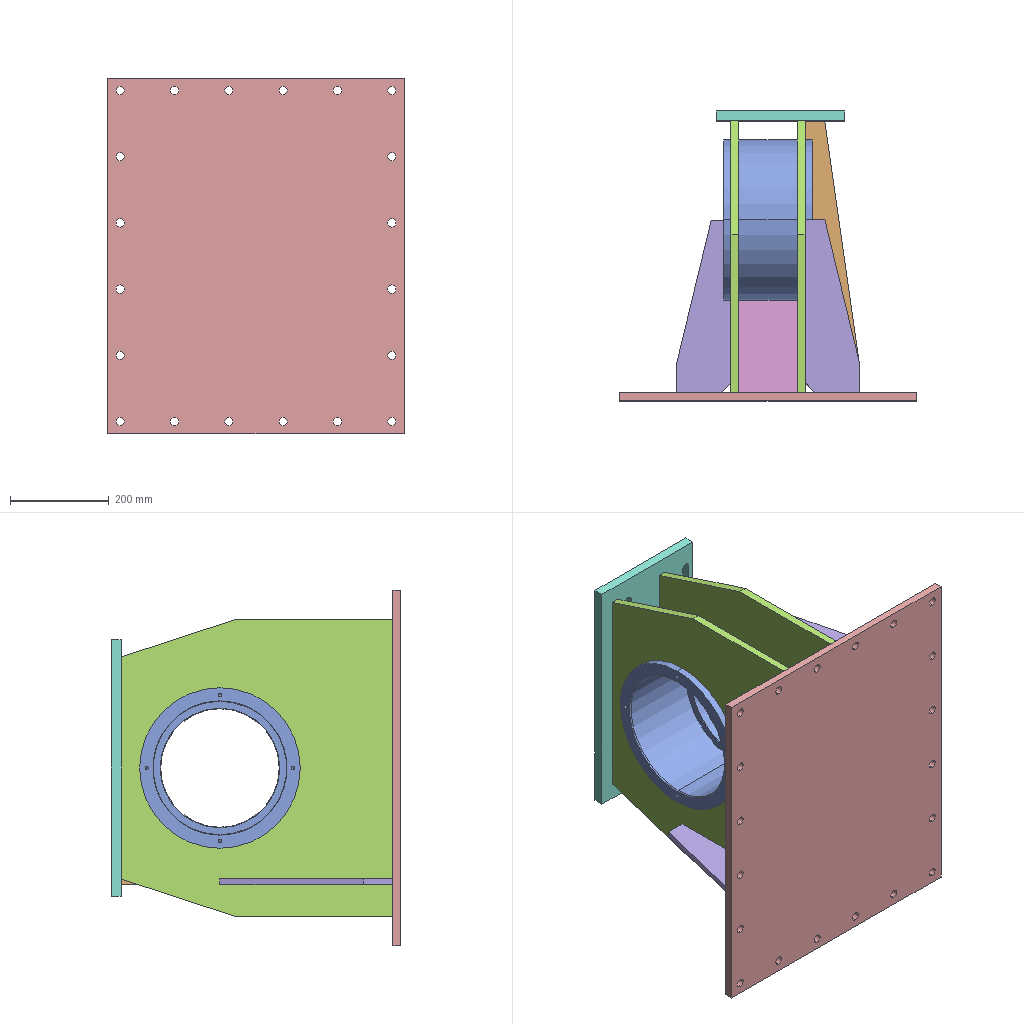Assembly | SolidWorks | 7 different items | 9 placed | box 600 x 586 x 720 mm
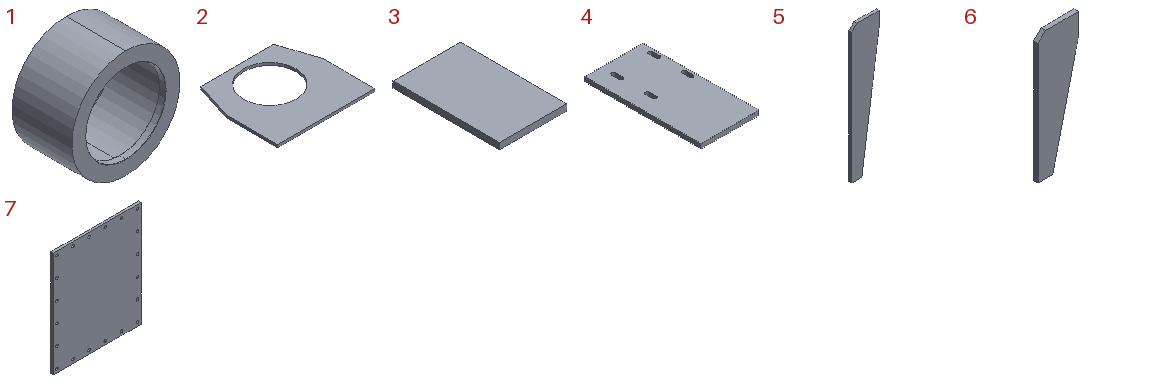Parts list (item | quantity | size | volume | features):
1 | x1 | 325 x 180 x 325 mm | 4860812 mm3 | features Chamfer 2, Extrusion 1, HoleWzd 1, ICE 1
2 | x2 | 600 x 550 x 16 mm | 3676677 mm3 | features Extrusion 1
3 | x1 | 118 x 187.5 x 11 mm | 243375 mm3 | features Extrusion 1
4 | x1 | 260 x 520 x 20 mm | 2637562 mm3 | features Extrusion 1, HoleWzd 1
5 | x1 | 110 x 12 x 550 mm | 517800 mm3 | features Chamfer 1, Extrusion 1
6 | x2 | 110 x 12 x 350 mm | 337800 mm3 | features Chamfer 1, Extrusion 1
7 | x1 | 600 x 16 x 720 mm | 6839366 mm3 | features Extrusion 1, HoleWzd 1
Mates (type | each side: item.copy, entity, surface, feature):
Coincident | 7.1 plane | assembly plane | 3 times
Coincident | 2.1 face plane Boss-Extrude1 | 2.2 face plane Boss-Extrude1 | 2 times
Coincident | 7.1 face plane Boss-Extrude1 | 2.1 face plane Boss-Extrude1
Coincident | 2.2 plane | assembly plane
Symmetric | 2.1 face plane Boss-Extrude1 | 2.2 face plane Boss-Extrude1 | assembly plane
DistanceDim | 2.1 face plane Boss-Extrude1 | 2.2 face plane Boss-Extrude1
Coincident | 4.1 face plane Boss-Extrude1 | 2.2 face plane Boss-Extrude1
DistanceDim | 2.2 face plane Boss-Extrude1 | 4.1 face plane Boss-Extrude1
Width | 4.1 face plane Boss-Extrude1 | 4.1 face plane Boss-Extrude1 | 7.1 face plane Boss-Extrude1 | 7.1 face plane Boss-Extrude1
Coincident | 5.1 face plane Boss-Extrude1 | 6.1 face plane Boss-Extrude1 | 2 times
Coincident | 7.1 face plane Boss-Extrude1 | 5.1 face plane Boss-Extrude1
Coincident | 2.1 face plane Boss-Extrude1 | 6.1 face plane Boss-Extrude1
DistanceDim | 5.1 face plane Boss-Extrude1 | 6.1 face plane Boss-Extrude1
Symmetric | 5.1 face plane Boss-Extrude1 | 6.1 face plane Boss-Extrude1 | assembly plane
Concentric | 1.1 face cylinder Boss-Extrude1 | 2.1 face cylinder Boss-Extrude1
DistanceDim | 2.2 face plane Boss-Extrude1 | 1.1 face plane Boss-Extrude1
Parallel | 1.1 plane | assembly plane
Coincident | 7.1 face plane Boss-Extrude1 | 6.2 face plane Boss-Extrude1
Coincident | 5.1 face plane Boss-Extrude1 | 6.2 face plane Boss-Extrude1
Coincident | 2.2 face plane Boss-Extrude1 | 6.2 face plane Boss-Extrude1
Coincident | 3.1 plane | assembly plane
Coincident | 7.1 face plane Boss-Extrude1 | 3.1 face plane Boss-Extrude1
Coincident | 2.1 face plane Boss-Extrude1 | 3.1 face plane Boss-Extrude1